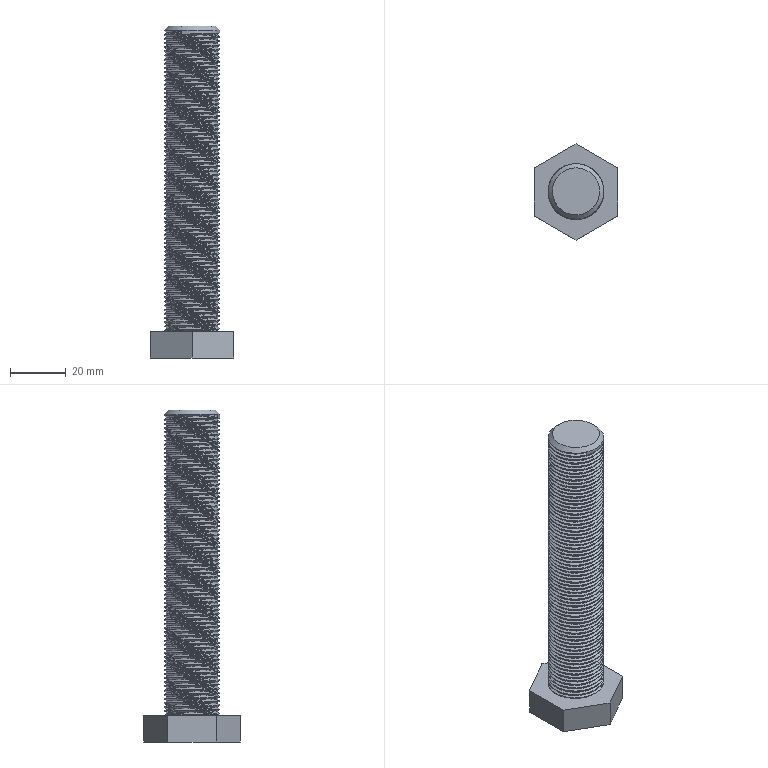Part | STEP file | 冲床-300配套压波_id1110_x_t | 1 solid | 15 faces | box 30 x 34.641 x 119.5 mm | volume 41362 mm3 | plane 10 | cylinder 2 | spline 2 | cone 1 | commonest cylinder face diameters 18.5 x1 20 x1